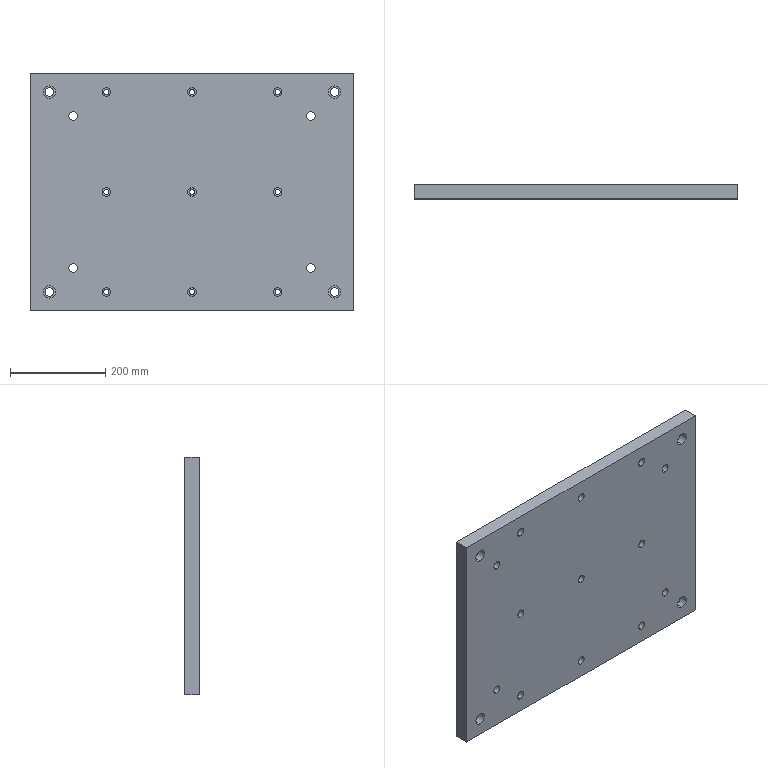Part | STEP file | OP10-016_lower plate (L)  | 1 solid | 99 faces | box 680 x 30 x 500 mm | volume 10067635 mm3 | cylinder 68 | plane 23 | cone 8 | commonest cylinder face diameters 18 x34 11 x18 26 x8 30 x8